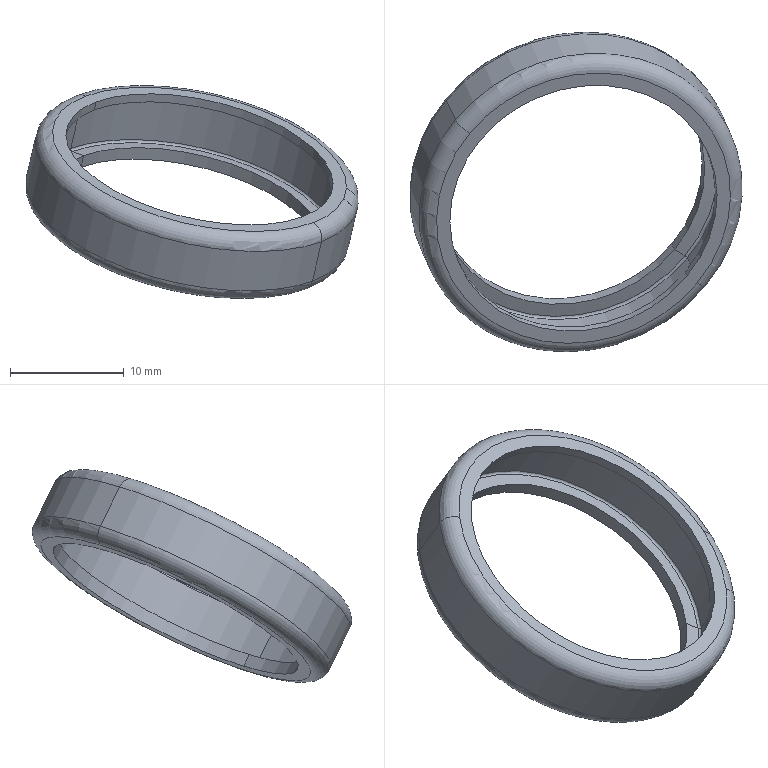Part | SolidWorks | features BaseBody 1 | 1 solid | 23 faces | box 29.254 x 28.081 x 18.745 mm | volume 719.848 mm3 | torus 10 | cylinder 8 | plane 3 | cone 2 | commonest cylinder face diameters 24 x4 27 x2 29 x2
STEP:
#1=CARTESIAN_POINT('',(1950.214,-223.457,971.31));
#2=VERTEX_POINT('',#1);
#3=CARTESIAN_POINT('',(1970.233,-236.588,960.184));
#4=VERTEX_POINT('',#3);
#5=CARTESIAN_POINT('',(1960.224,-230.022,965.747));
#6=DIRECTION('',(0.2015,-0.436,0.8771));
#7=DIRECTION('',(0.9077,0.4197,0.0001618));
#8=AXIS2_PLACEMENT_3D('',#5,#6,#7);
#9=CIRCLE('',#8,13.2);
#10=EDGE_CURVE('',#2,#4,#9,.T.);
#11=ORIENTED_EDGE('',*,*,#10,.F.);
#12=CARTESIAN_POINT('',(1948.967,-222.243,970.717));
#13=VERTEX_POINT('',#12);
#14=CARTESIAN_POINT('',(1949.952,-222.89,970.17));
#15=DIRECTION('',(0.62,0.75,0.2304));
#16=DIRECTION('',(0.7583,-0.4974,-0.4214));
#17=AXIS2_PLACEMENT_3D('',#14,#15,#16);
#18=CIRCLE('',#17,1.3);
#19=EDGE_CURVE('',#13,#2,#18,.T.);
#20=ORIENTED_EDGE('',*,*,#19,.F.);
#21=CARTESIAN_POINT('',(1970.957,-236.668,958.496));
#22=VERTEX_POINT('',#21);
#23=CARTESIAN_POINT('',(1959.962,-229.456,964.607));
#24=DIRECTION('',(0.2015,-0.436,0.8771));
#25=DIRECTION('',(0.9077,0.4197,0.0001618));
#26=AXIS2_PLACEMENT_3D('',#23,#24,#25);
#27=CIRCLE('',#26,14.5);
#28=EDGE_CURVE('',#13,#22,#27,.T.);
#29=ORIENTED_EDGE('',*,*,#28,.T.);
#30=CARTESIAN_POINT('',(1969.971,-236.021,959.044));
#31=DIRECTION('',(0.62,0.75,0.2304));
#32=DIRECTION('',(0.7583,-0.4974,-0.4214));
#33=AXIS2_PLACEMENT_3D('',#30,#31,#32);
#34=CIRCLE('',#33,1.3);
#35=EDGE_CURVE('',#4,#22,#34,.T.);
#36=ORIENTED_EDGE('',*,*,#35,.F.);
#37=EDGE_LOOP('',(#11,#20,#29,#36));
#38=FACE_OUTER_BOUND('',#37,.T.);
#39=CARTESIAN_POINT('',(1959.962,-229.456,964.607));
#40=DIRECTION('',(0.2015,-0.436,0.8771));
#41=DIRECTION('',(0.7583,-0.4974,-0.4214));
#42=AXIS2_PLACEMENT_3D('',#39,#40,#41);
#43=TOROIDAL_SURFACE('',#42,13.2,1.3);
#44=ADVANCED_FACE('',(#38),#43,.T.);
#45=CARTESIAN_POINT('',(1960.224,-230.022,965.747));
#46=DIRECTION('',(0.2015,-0.436,0.8771));
#47=DIRECTION('',(0.9077,0.4197,0.0001618));
#48=AXIS2_PLACEMENT_3D('',#45,#46,#47);
#49=CIRCLE('',#48,13.2);
#50=EDGE_CURVE('',#4,#2,#49,.T.);
#51=ORIENTED_EDGE('',*,*,#50,.F.);
#52=ORIENTED_EDGE('',*,*,#35,.T.);
#53=CARTESIAN_POINT('',(1959.962,-229.456,964.607));
#54=DIRECTION('',(0.2015,-0.436,0.8771));
#55=DIRECTION('',(0.9077,0.4197,0.0001618));
#56=AXIS2_PLACEMENT_3D('',#53,#54,#55);
#57=CIRCLE('',#56,14.5);
#58=EDGE_CURVE('',#22,#13,#57,.T.);
#59=ORIENTED_EDGE('',*,*,#58,.T.);
#60=ORIENTED_EDGE('',*,*,#19,.T.);
#61=EDGE_LOOP('',(#51,#52,#59,#60));
#62=FACE_OUTER_BOUND('',#61,.T.);
#63=CARTESIAN_POINT('',(1959.962,-229.456,964.607));
#64=DIRECTION('',(0.2015,-0.436,0.8771));
#65=DIRECTION('',(0.7583,-0.4974,-0.4214));
#66=AXIS2_PLACEMENT_3D('',#63,#64,#65);
#67=TOROIDAL_SURFACE('',#66,13.2,1.3);
#68=ADVANCED_FACE('',(#62),#67,.T.);
#69=ORIENTED_EDGE('',*,*,#28,.F.);
#70=CARTESIAN_POINT('',(1948.171,-220.521,967.253));
#71=VERTEX_POINT('',#70);
#72=CARTESIAN_POINT('',(1948.569,-221.382,968.985));
#73=DIRECTION('',(-0.2015,0.436,-0.8771));
#74=VECTOR('',#73,1000.);
#75=LINE('',#72,#74);
#76=EDGE_CURVE('',#13,#71,#75,.T.);
#77=ORIENTED_EDGE('',*,*,#76,.T.);
#78=CARTESIAN_POINT('',(1970.161,-234.946,955.031));
#79=VERTEX_POINT('',#78);
#80=CARTESIAN_POINT('',(1959.166,-227.733,961.142));
#81=DIRECTION('',(0.2015,-0.436,0.8771));
#82=DIRECTION('',(0.9077,0.4197,0.0001618));
#83=AXIS2_PLACEMENT_3D('',#80,#81,#82);
#84=CIRCLE('',#83,14.5);
#85=EDGE_CURVE('',#71,#79,#84,.T.);
#86=ORIENTED_EDGE('',*,*,#85,.T.);
#87=CARTESIAN_POINT('',(1970.559,-235.807,956.763));
#88=DIRECTION('',(0.2015,-0.436,0.8771));
#89=VECTOR('',#88,1000.);
#90=LINE('',#87,#89);
#91=EDGE_CURVE('',#79,#22,#90,.T.);
#92=ORIENTED_EDGE('',*,*,#91,.T.);
#93=EDGE_LOOP('',(#69,#77,#86,#92));
#94=FACE_OUTER_BOUND('',#93,.T.);
#95=CARTESIAN_POINT('',(1959.564,-228.595,962.874));
#96=DIRECTION('',(0.2015,-0.436,0.8771));
#97=DIRECTION('',(0.7583,-0.4974,-0.4214));
#98=AXIS2_PLACEMENT_3D('',#95,#96,#97);
#99=CYLINDRICAL_SURFACE('',#98,14.5);
#100=ADVANCED_FACE('',(#94),#99,.T.);
#101=ORIENTED_EDGE('',*,*,#58,.F.);
#102=ORIENTED_EDGE('',*,*,#91,.F.);
#103=CARTESIAN_POINT('',(1959.166,-227.733,961.142));
#104=DIRECTION('',(0.2015,-0.436,0.8771));
#105=DIRECTION('',(0.9077,0.4197,0.0001618));
#106=AXIS2_PLACEMENT_3D('',#103,#104,#105);
#107=CIRCLE('',#106,14.5);
#108=EDGE_CURVE('',#79,#71,#107,.T.);
#109=ORIENTED_EDGE('',*,*,#108,.T.);
#110=ORIENTED_EDGE('',*,*,#76,.F.);
#111=EDGE_LOOP('',(#101,#102,#109,#110));
#112=FACE_OUTER_BOUND('',#111,.T.);
#113=CARTESIAN_POINT('',(1959.564,-228.595,962.874));
#114=DIRECTION('',(0.2015,-0.436,0.8771));
#115=DIRECTION('',(0.7583,-0.4974,-0.4214));
#116=AXIS2_PLACEMENT_3D('',#113,#114,#115);
#117=CYLINDRICAL_SURFACE('',#116,14.5);
#118=ADVANCED_FACE('',(#112),#117,.T.);
#119=ORIENTED_EDGE('',*,*,#85,.F.);
#120=CARTESIAN_POINT('',(1948.895,-220.601,965.565));
#121=VERTEX_POINT('',#120);
#122=CARTESIAN_POINT('',(1949.157,-221.168,966.705));
#123=DIRECTION('',(-0.62,-0.75,-0.2304));
#124=DIRECTION('',(0.7583,-0.4974,-0.4214));
#125=AXIS2_PLACEMENT_3D('',#122,#123,#124);
#126=CIRCLE('',#125,1.3);
#127=EDGE_CURVE('',#71,#121,#126,.T.);
#128=ORIENTED_EDGE('',*,*,#127,.T.);
#129=CARTESIAN_POINT('',(1968.913,-233.732,954.439));
#130=VERTEX_POINT('',#129);
#131=CARTESIAN_POINT('',(1958.904,-227.167,960.002));
#132=DIRECTION('',(0.2015,-0.436,0.8771));
#133=DIRECTION('',(0.9077,0.4197,0.0001618));
#134=AXIS2_PLACEMENT_3D('',#131,#132,#133);
#135=CIRCLE('',#134,13.2);
#136=EDGE_CURVE('',#121,#130,#135,.T.);
#137=ORIENTED_EDGE('',*,*,#136,.T.);
#138=CARTESIAN_POINT('',(1969.175,-234.299,955.579));
#139=DIRECTION('',(-0.62,-0.75,-0.2304));
#140=DIRECTION('',(0.7583,-0.4974,-0.4214));
#141=AXIS2_PLACEMENT_3D('',#138,#139,#140);
#142=CIRCLE('',#141,1.3);
#143=EDGE_CURVE('',#130,#79,#142,.T.);
#144=ORIENTED_EDGE('',*,*,#143,.T.);
#145=EDGE_LOOP('',(#119,#128,#137,#144));
#146=FACE_OUTER_BOUND('',#145,.T.);
#147=CARTESIAN_POINT('',(1959.166,-227.733,961.142));
#148=DIRECTION('',(0.2015,-0.436,0.8771));
#149=DIRECTION('',(0.7583,-0.4974,-0.4214));
#150=AXIS2_PLACEMENT_3D('',#147,#148,#149);
#151=TOROIDAL_SURFACE('',#150,13.2,1.3);
#152=ADVANCED_FACE('',(#146),#151,.T.);
#153=ORIENTED_EDGE('',*,*,#108,.F.);
#154=ORIENTED_EDGE('',*,*,#143,.F.);
#155=CARTESIAN_POINT('',(1958.904,-227.167,960.002));
#156=DIRECTION('',(0.2015,-0.436,0.8771));
#157=DIRECTION('',(0.9077,0.4197,0.0001618));
#158=AXIS2_PLACEMENT_3D('',#155,#156,#157);
#159=CIRCLE('',#158,13.2);
#160=EDGE_CURVE('',#130,#121,#159,.T.);
#161=ORIENTED_EDGE('',*,*,#160,.T.);
#162=ORIENTED_EDGE('',*,*,#127,.F.);
#163=EDGE_LOOP('',(#153,#154,#161,#162));
#164=FACE_OUTER_BOUND('',#163,.T.);
#165=CARTESIAN_POINT('',(1959.166,-227.733,961.142));
#166=DIRECTION('',(0.2015,-0.436,0.8771));
#167=DIRECTION('',(0.7583,-0.4974,-0.4214));
#168=AXIS2_PLACEMENT_3D('',#165,#166,#167);
#169=TOROIDAL_SURFACE('',#168,13.2,1.3);
#170=ADVANCED_FACE('',(#164),#169,.T.);
#171=CARTESIAN_POINT('',(1949.805,-221.198,965.059));
#172=VERTEX_POINT('',#171);
#173=CARTESIAN_POINT('',(1968.004,-233.135,954.945));
#174=VERTEX_POINT('',#173);
#175=CARTESIAN_POINT('',(1958.904,-227.167,960.002));
#176=DIRECTION('',(0.2015,-0.436,0.8771));
#177=DIRECTION('',(0.9077,0.4197,0.0001618));
#178=AXIS2_PLACEMENT_3D('',#175,#176,#177);
#179=CIRCLE('',#178,12.);
#180=EDGE_CURVE('',#172,#174,#179,.T.);
#181=ORIENTED_EDGE('',*,*,#180,.F.);
#182=CARTESIAN_POINT('',(1950.036,-221.699,966.068));
#183=VERTEX_POINT('',#182);
#184=CARTESIAN_POINT('',(1950.465,-222.626,967.932));
#185=DIRECTION('',(0.2015,-0.436,0.8771));
#186=VECTOR('',#185,1000.);
#187=LINE('',#184,#186);
#188=EDGE_CURVE('',#172,#183,#187,.T.);
#189=ORIENTED_EDGE('',*,*,#188,.T.);
#190=CARTESIAN_POINT('',(1968.235,-233.637,955.953));
#191=VERTEX_POINT('',#190);
#192=CARTESIAN_POINT('',(1959.136,-227.668,961.01));
#193=DIRECTION('',(0.2015,-0.436,0.8771));
#194=DIRECTION('',(0.9077,0.4197,0.0001618));
#195=AXIS2_PLACEMENT_3D('',#192,#193,#194);
#196=CIRCLE('',#195,12.);
#197=EDGE_CURVE('',#183,#191,#196,.T.);
#198=ORIENTED_EDGE('',*,*,#197,.T.);
#199=CARTESIAN_POINT('',(1968.663,-234.563,957.817));
#200=DIRECTION('',(-0.2015,0.436,-0.8771));
#201=VECTOR('',#200,1000.);
#202=LINE('',#199,#201);
#203=EDGE_CURVE('',#191,#174,#202,.T.);
#204=ORIENTED_EDGE('',*,*,#203,.T.);
#205=EDGE_LOOP('',(#181,#189,#198,#204));
#206=FACE_OUTER_BOUND('',#205,.T.);
#207=CARTESIAN_POINT('',(1959.564,-228.595,962.874));
#208=DIRECTION('',(0.2015,-0.436,0.8771));
#209=DIRECTION('',(0.7583,-0.4974,-0.4214));
#210=AXIS2_PLACEMENT_3D('',#207,#208,#209);
#211=CYLINDRICAL_SURFACE('',#210,12.);
#212=ADVANCED_FACE('',(#206),#211,.F.);
#213=CARTESIAN_POINT('',(1958.904,-227.167,960.002));
#214=DIRECTION('',(0.2015,-0.436,0.8771));
#215=DIRECTION('',(0.9077,0.4197,0.0001618));
#216=AXIS2_PLACEMENT_3D('',#213,#214,#215);
#217=CIRCLE('',#216,12.);
#218=EDGE_CURVE('',#174,#172,#217,.T.);
#219=ORIENTED_EDGE('',*,*,#218,.F.);
#220=ORIENTED_EDGE('',*,*,#203,.F.);
#221=CARTESIAN_POINT('',(1959.136,-227.668,961.01));
#222=DIRECTION('',(0.2015,-0.436,0.8771));
#223=DIRECTION('',(0.9077,0.4197,0.0001618));
#224=AXIS2_PLACEMENT_3D('',#221,#222,#223);
#225=CIRCLE('',#224,12.);
#226=EDGE_CURVE('',#191,#183,#225,.T.);
#227=ORIENTED_EDGE('',*,*,#226,.T.);
#228=ORIENTED_EDGE('',*,*,#188,.F.);
#229=EDGE_LOOP('',(#219,#220,#227,#228));
#230=FACE_OUTER_BOUND('',#229,.T.);
#231=CARTESIAN_POINT('',(1959.564,-228.595,962.874));
#232=DIRECTION('',(0.2015,-0.436,0.8771));
#233=DIRECTION('',(0.7583,-0.4974,-0.4214));
#234=AXIS2_PLACEMENT_3D('',#231,#232,#233);
#235=CYLINDRICAL_SURFACE('',#234,12.);
#236=ADVANCED_FACE('',(#230),#235,.F.);
#237=ORIENTED_EDGE('',*,*,#197,.F.);
#238=CARTESIAN_POINT('',(1949.034,-220.982,966.429));
#239=VERTEX_POINT('',#238);
#240=CARTESIAN_POINT('',(1949.535,-221.341,966.248));
#241=DIRECTION('',(0.7803,-0.5585,-0.2815));
#242=VECTOR('',#241,1000.);
#243=LINE('',#240,#242);
#244=EDGE_CURVE('',#239,#183,#243,.T.);
#245=ORIENTED_EDGE('',*,*,#244,.F.);
#246=CARTESIAN_POINT('',(1969.158,-234.182,955.245));
#247=VERTEX_POINT('',#246);
#248=CARTESIAN_POINT('',(1959.096,-227.582,960.837));
#249=DIRECTION('',(0.2015,-0.436,0.8771));
#250=DIRECTION('',(0.9077,0.4197,0.0001618));
#251=AXIS2_PLACEMENT_3D('',#248,#249,#250);
#252=CIRCLE('',#251,13.269);
#253=EDGE_CURVE('',#239,#247,#252,.T.);
#254=ORIENTED_EDGE('',*,*,#253,.T.);
#255=CARTESIAN_POINT('',(1968.697,-233.909,955.599));
#256=DIRECTION('',(0.7183,-0.4244,-0.5514));
#257=VECTOR('',#256,1000.);
#258=LINE('',#255,#257);
#259=EDGE_CURVE('',#191,#247,#258,.T.);
#260=ORIENTED_EDGE('',*,*,#259,.F.);
#261=EDGE_LOOP('',(#237,#245,#254,#260));
#262=FACE_OUTER_BOUND('',#261,.T.);
#263=CARTESIAN_POINT('',(1959.136,-227.668,961.01));
#264=DIRECTION('',(-0.2015,0.436,-0.8771));
#265=DIRECTION('',(0.7583,-0.4974,-0.4214));
#266=AXIS2_PLACEMENT_3D('',#263,#264,#265);
#267=CONICAL_SURFACE('',#266,12.,1.416);
#268=ADVANCED_FACE('',(#262),#267,.T.);
#269=ORIENTED_EDGE('',*,*,#226,.F.);
#270=ORIENTED_EDGE('',*,*,#259,.T.);
#271=CARTESIAN_POINT('',(1959.096,-227.582,960.837));
#272=DIRECTION('',(0.2015,-0.436,0.8771));
#273=DIRECTION('',(0.9077,0.4197,0.0001618));
#274=AXIS2_PLACEMENT_3D('',#271,#272,#273);
#275=CIRCLE('',#274,13.269);
#276=EDGE_CURVE('',#247,#239,#275,.T.);
#277=ORIENTED_EDGE('',*,*,#276,.T.);
#278=ORIENTED_EDGE('',*,*,#244,.T.);
#279=EDGE_LOOP('',(#269,#270,#277,#278));
#280=FACE_OUTER_BOUND('',#279,.T.);
#281=CARTESIAN_POINT('',(1959.136,-227.668,961.01));
#282=DIRECTION('',(-0.2015,0.436,-0.8771));
#283=DIRECTION('',(0.7583,-0.4974,-0.4214));
#284=AXIS2_PLACEMENT_3D('',#281,#282,#283);
#285=CONICAL_SURFACE('',#284,12.,1.416);
#286=ADVANCED_FACE('',(#280),#285,.T.);
#287=ORIENTED_EDGE('',*,*,#253,.F.);
#288=CARTESIAN_POINT('',(1948.899,-220.953,966.7));
#289=VERTEX_POINT('',#288);
#290=CARTESIAN_POINT('',(1949.051,-221.053,966.616));
#291=DIRECTION('',(0.62,0.75,0.2304));
#292=DIRECTION('',(0.7583,-0.4974,-0.4214));
#293=AXIS2_PLACEMENT_3D('',#290,#291,#292);
#294=CIRCLE('',#293,0.2);
#295=EDGE_CURVE('',#239,#289,#294,.T.);
#296=ORIENTED_EDGE('',*,*,#295,.T.);
#297=CARTESIAN_POINT('',(1969.373,-234.383,955.321));
#298=VERTEX_POINT('',#297);
#299=CARTESIAN_POINT('',(1959.136,-227.668,961.01));
#300=DIRECTION('',(0.2015,-0.436,0.8771));
#301=DIRECTION('',(0.9077,0.4197,0.0001618));
#302=AXIS2_PLACEMENT_3D('',#299,#300,#301);
#303=CIRCLE('',#302,13.5);
#304=EDGE_CURVE('',#289,#298,#303,.T.);
#305=ORIENTED_EDGE('',*,*,#304,.T.);
#306=CARTESIAN_POINT('',(1969.221,-234.283,955.405));
#307=DIRECTION('',(0.62,0.75,0.2304));
#308=DIRECTION('',(0.7583,-0.4974,-0.4214));
#309=AXIS2_PLACEMENT_3D('',#306,#307,#308);
#310=CIRCLE('',#309,0.2);
#311=EDGE_CURVE('',#298,#247,#310,.T.);
#312=ORIENTED_EDGE('',*,*,#311,.T.);
#313=EDGE_LOOP('',(#287,#296,#305,#312));
#314=FACE_OUTER_BOUND('',#313,.T.);
#315=CARTESIAN_POINT('',(1959.136,-227.668,961.01));
#316=DIRECTION('',(0.2015,-0.436,0.8771));
#317=DIRECTION('',(0.7583,-0.4974,-0.4214));
#318=AXIS2_PLACEMENT_3D('',#315,#316,#317);
#319=TOROIDAL_SURFACE('',#318,13.3,0.2);
#320=ADVANCED_FACE('',(#314),#319,.F.);
#321=ORIENTED_EDGE('',*,*,#276,.F.);
#322=ORIENTED_EDGE('',*,*,#311,.F.);
#323=CARTESIAN_POINT('',(1959.136,-227.668,961.01));
#324=DIRECTION('',(0.2015,-0.436,0.8771));
#325=DIRECTION('',(0.9077,0.4197,0.0001618));
#326=AXIS2_PLACEMENT_3D('',#323,#324,#325);
#327=CIRCLE('',#326,13.5);
#328=EDGE_CURVE('',#298,#289,#327,.T.);
#329=ORIENTED_EDGE('',*,*,#328,.T.);
#330=ORIENTED_EDGE('',*,*,#295,.F.);
#331=EDGE_LOOP('',(#321,#322,#329,#330));
#332=FACE_OUTER_BOUND('',#331,.T.);
#333=CARTESIAN_POINT('',(1959.136,-227.668,961.01));
#334=DIRECTION('',(0.2015,-0.436,0.8771));
#335=DIRECTION('',(0.7583,-0.4974,-0.4214));
#336=AXIS2_PLACEMENT_3D('',#333,#334,#335);
#337=TOROIDAL_SURFACE('',#336,13.3,0.2);
#338=ADVANCED_FACE('',(#332),#337,.F.);
#339=ORIENTED_EDGE('',*,*,#304,.F.);
#340=CARTESIAN_POINT('',(1949.685,-222.654,970.121));
#341=VERTEX_POINT('',#340);
#342=CARTESIAN_POINT('',(1949.292,-221.803,968.41));
#343=DIRECTION('',(-0.2015,0.436,-0.8771));
#344=VECTOR('',#343,1000.);
#345=LINE('',#342,#344);
#346=EDGE_CURVE('',#341,#289,#345,.T.);
#347=ORIENTED_EDGE('',*,*,#346,.F.);
#348=CARTESIAN_POINT('',(1970.158,-236.083,958.742));
#349=VERTEX_POINT('',#348);
#350=CARTESIAN_POINT('',(1959.922,-229.368,964.431));
#351=DIRECTION('',(0.2015,-0.436,0.8771));
#352=DIRECTION('',(0.9077,0.4197,0.0001618));
#353=AXIS2_PLACEMENT_3D('',#350,#351,#352);
#354=CIRCLE('',#353,13.5);
#355=EDGE_CURVE('',#341,#349,#354,.T.);
#356=ORIENTED_EDGE('',*,*,#355,.T.);
#357=CARTESIAN_POINT('',(1969.765,-235.233,957.031));
#358=DIRECTION('',(0.2015,-0.436,0.8771));
#359=VECTOR('',#358,1000.);
#360=LINE('',#357,#359);
#361=EDGE_CURVE('',#298,#349,#360,.T.);
#362=ORIENTED_EDGE('',*,*,#361,.F.);
#363=EDGE_LOOP('',(#339,#347,#356,#362));
#364=FACE_OUTER_BOUND('',#363,.T.);
#365=CARTESIAN_POINT('',(1959.564,-228.595,962.874));
#366=DIRECTION('',(0.2015,-0.436,0.8771));
#367=DIRECTION('',(0.7583,-0.4974,-0.4214));
#368=AXIS2_PLACEMENT_3D('',#365,#366,#367);
#369=CYLINDRICAL_SURFACE('',#368,13.5);
#370=ADVANCED_FACE('',(#364),#369,.F.);
#371=ORIENTED_EDGE('',*,*,#328,.F.);
#372=ORIENTED_EDGE('',*,*,#361,.T.);
#373=CARTESIAN_POINT('',(1959.922,-229.368,964.431));
#374=DIRECTION('',(0.2015,-0.436,0.8771));
#375=DIRECTION('',(0.9077,0.4197,0.0001618));
#376=AXIS2_PLACEMENT_3D('',#373,#374,#375);
#377=CIRCLE('',#376,13.5);
#378=EDGE_CURVE('',#349,#341,#377,.T.);
#379=ORIENTED_EDGE('',*,*,#378,.T.);
#380=ORIENTED_EDGE('',*,*,#346,.T.);
#381=EDGE_LOOP('',(#371,#372,#379,#380));
#382=FACE_OUTER_BOUND('',#381,.T.);
#383=CARTESIAN_POINT('',(1959.564,-228.595,962.874));
#384=DIRECTION('',(0.2015,-0.436,0.8771));
#385=DIRECTION('',(0.7583,-0.4974,-0.4214));
#386=AXIS2_PLACEMENT_3D('',#383,#384,#385);
#387=CYLINDRICAL_SURFACE('',#386,13.5);
#388=ADVANCED_FACE('',(#382),#387,.F.);
#389=ORIENTED_EDGE('',*,*,#355,.F.);
#390=CARTESIAN_POINT('',(1949.585,-222.635,970.329));
#391=VERTEX_POINT('',#390);
#392=CARTESIAN_POINT('',(1948.983,-221.992,969.855));
#393=DIRECTION('',(-0.62,-0.75,-0.2304));
#394=DIRECTION('',(0.7583,-0.4974,-0.4214));
#395=AXIS2_PLACEMENT_3D('',#392,#393,#394);
#396=CIRCLE('',#395,1.);
#397=EDGE_CURVE('',#341,#391,#396,.T.);
#398=ORIENTED_EDGE('',*,*,#397,.T.);
#399=CARTESIAN_POINT('',(1970.321,-236.237,958.805));
#400=VERTEX_POINT('',#399);
#401=CARTESIAN_POINT('',(1959.953,-229.436,964.567));
#402=DIRECTION('',(0.2015,-0.436,0.8771));
#403=DIRECTION('',(0.9077,0.4197,0.0001618));
#404=AXIS2_PLACEMENT_3D('',#401,#402,#403);
#405=CIRCLE('',#404,13.673);
#406=EDGE_CURVE('',#391,#400,#405,.T.);
#407=ORIENTED_EDGE('',*,*,#406,.T.);
#408=CARTESIAN_POINT('',(1970.593,-236.167,957.845));
#409=DIRECTION('',(-0.62,-0.75,-0.2304));
#410=DIRECTION('',(0.7583,-0.4974,-0.4214));
#411=AXIS2_PLACEMENT_3D('',#408,#409,#410);
#412=CIRCLE('',#411,1.);
#413=EDGE_CURVE('',#400,#349,#412,.T.);
#414=ORIENTED_EDGE('',*,*,#413,.T.);
#415=EDGE_LOOP('',(#389,#398,#407,#414));
#416=FACE_OUTER_BOUND('',#415,.T.);
#417=CARTESIAN_POINT('',(1959.788,-229.08,963.85));
#418=DIRECTION('',(0.2015,-0.436,0.8771));
#419=DIRECTION('',(0.7583,-0.4974,-0.4214));
#420=AXIS2_PLACEMENT_3D('',#417,#418,#419);
#421=TOROIDAL_SURFACE('',#420,14.249,1.);
#422=ADVANCED_FACE('',(#416),#421,.T.);
#423=ORIENTED_EDGE('',*,*,#378,.F.);
#424=ORIENTED_EDGE('',*,*,#413,.F.);
#425=CARTESIAN_POINT('',(1959.953,-229.436,964.567));
#426=DIRECTION('',(0.2015,-0.436,0.8771));
#427=DIRECTION('',(0.9077,0.4197,0.0001618));
#428=AXIS2_PLACEMENT_3D('',#425,#426,#427);
#429=CIRCLE('',#428,13.673);
#430=EDGE_CURVE('',#400,#391,#429,.T.);
#431=ORIENTED_EDGE('',*,*,#430,.T.);
#432=ORIENTED_EDGE('',*,*,#397,.F.);
#433=EDGE_LOOP('',(#423,#424,#431,#432));
#434=FACE_OUTER_BOUND('',#433,.T.);
#435=CARTESIAN_POINT('',(1959.788,-229.08,963.85));
#436=DIRECTION('',(0.2015,-0.436,0.8771));
#437=DIRECTION('',(0.7583,-0.4974,-0.4214));
#438=AXIS2_PLACEMENT_3D('',#435,#436,#437);
#439=TOROIDAL_SURFACE('',#438,14.249,1.);
#440=ADVANCED_FACE('',(#434),#439,.T.);
#441=ORIENTED_EDGE('',*,*,#406,.F.);
#442=CARTESIAN_POINT('',(1949.826,-222.959,970.735));
#443=VERTEX_POINT('',#442);
#444=CARTESIAN_POINT('',(1949.765,-222.828,970.471));
#445=DIRECTION('',(0.62,0.75,0.2304));
#446=DIRECTION('',(0.7583,-0.4974,-0.4214));
#447=AXIS2_PLACEMENT_3D('',#444,#445,#446);
#448=CIRCLE('',#447,0.3);
#449=EDGE_CURVE('',#391,#443,#448,.T.);
#450=ORIENTED_EDGE('',*,*,#449,.T.);
#451=CARTESIAN_POINT('',(1970.299,-236.388,959.356));
#452=VERTEX_POINT('',#451);
#453=CARTESIAN_POINT('',(1960.063,-229.674,965.045));
#454=DIRECTION('',(0.2015,-0.436,0.8771));
#455=DIRECTION('',(0.9077,0.4197,0.0001618));
#456=AXIS2_PLACEMENT_3D('',#453,#454,#455);
#457=CIRCLE('',#456,13.5);
#458=EDGE_CURVE('',#443,#452,#457,.T.);
#459=ORIENTED_EDGE('',*,*,#458,.T.);
#460=CARTESIAN_POINT('',(1970.239,-236.258,959.093));
#461=DIRECTION('',(0.62,0.75,0.2304));
#462=DIRECTION('',(0.7583,-0.4974,-0.4214));
#463=AXIS2_PLACEMENT_3D('',#460,#461,#462);
#464=CIRCLE('',#463,0.3);
#465=EDGE_CURVE('',#452,#400,#464,.T.);
#466=ORIENTED_EDGE('',*,*,#465,.T.);
#467=EDGE_LOOP('',(#441,#450,#459,#466));
#468=FACE_OUTER_BOUND('',#467,.T.);
#469=CARTESIAN_POINT('',(1960.002,-229.543,964.782));
#470=DIRECTION('',(0.2015,-0.436,0.8771));
#471=DIRECTION('',(0.7583,-0.4974,-0.4214));
#472=AXIS2_PLACEMENT_3D('',#469,#470,#471);
#473=TOROIDAL_SURFACE('',#472,13.5,0.3);
#474=ADVANCED_FACE('',(#468),#473,.F.);
#475=ORIENTED_EDGE('',*,*,#430,.F.);
#476=ORIENTED_EDGE('',*,*,#465,.F.);
#477=CARTESIAN_POINT('',(1960.063,-229.674,965.045));
#478=DIRECTION('',(0.2015,-0.436,0.8771));
#479=DIRECTION('',(0.9077,0.4197,0.0001618));
#480=AXIS2_PLACEMENT_3D('',#477,#478,#479);
#481=CIRCLE('',#480,13.5);
#482=EDGE_CURVE('',#452,#443,#481,.T.);
#483=ORIENTED_EDGE('',*,*,#482,.T.);
#484=ORIENTED_EDGE('',*,*,#449,.F.);
#485=EDGE_LOOP('',(#475,#476,#483,#484));
#486=FACE_OUTER_BOUND('',#485,.T.);
#487=CARTESIAN_POINT('',(1960.002,-229.543,964.782));
#488=DIRECTION('',(0.2015,-0.436,0.8771));
#489=DIRECTION('',(0.7583,-0.4974,-0.4214));
#490=AXIS2_PLACEMENT_3D('',#487,#488,#489);
#491=TOROIDAL_SURFACE('',#490,13.5,0.3);
#492=ADVANCED_FACE('',(#486),#491,.F.);
#493=CARTESIAN_POINT('',(1950.963,-223.705,970.102));
#494=VERTEX_POINT('',#493);
#495=CARTESIAN_POINT('',(1969.162,-235.642,959.988));
#496=VERTEX_POINT('',#495);
#497=CARTESIAN_POINT('',(1960.063,-229.674,965.045));
#498=DIRECTION('',(0.2015,-0.436,0.8771));
#499=DIRECTION('',(0.9077,0.4197,0.0001618));
#500=AXIS2_PLACEMENT_3D('',#497,#498,#499);
#501=CIRCLE('',#500,12.);
#502=EDGE_CURVE('',#494,#496,#501,.T.);
#503=ORIENTED_EDGE('',*,*,#502,.F.);
#504=CARTESIAN_POINT('',(1951.124,-224.054,970.804));
#505=VERTEX_POINT('',#504);
#506=CARTESIAN_POINT('',(1950.465,-222.626,967.932));
#507=DIRECTION('',(-0.2015,0.436,-0.8771));
#508=VECTOR('',#507,1000.);
#509=LINE('',#506,#508);
#510=EDGE_CURVE('',#505,#494,#509,.T.);
#511=ORIENTED_EDGE('',*,*,#510,.F.);
#512=CARTESIAN_POINT('',(1969.323,-235.991,960.69));
#513=VERTEX_POINT('',#512);
#514=CARTESIAN_POINT('',(1960.224,-230.022,965.747));
#515=DIRECTION('',(0.2015,-0.436,0.8771));
#516=DIRECTION('',(0.9077,0.4197,0.0001618));
#517=AXIS2_PLACEMENT_3D('',#514,#515,#516);
#518=CIRCLE('',#517,12.);
#519=EDGE_CURVE('',#505,#513,#518,.T.);
#520=ORIENTED_EDGE('',*,*,#519,.T.);
#521=CARTESIAN_POINT('',(1968.663,-234.563,957.817));
#522=DIRECTION('',(0.2015,-0.436,0.8771));
#523=VECTOR('',#522,1000.);
#524=LINE('',#521,#523);
#525=EDGE_CURVE('',#496,#513,#524,.T.);
#526=ORIENTED_EDGE('',*,*,#525,.F.);
#527=EDGE_LOOP('',(#503,#511,#520,#526));
#528=FACE_OUTER_BOUND('',#527,.T.);
#529=CARTESIAN_POINT('',(1959.564,-228.595,962.874));
#530=DIRECTION('',(0.2015,-0.436,0.8771));
#531=DIRECTION('',(0.7583,-0.4974,-0.4214));
#532=AXIS2_PLACEMENT_3D('',#529,#530,#531);
#533=CYLINDRICAL_SURFACE('',#532,12.);
#534=ADVANCED_FACE('',(#528),#533,.F.);
#535=CARTESIAN_POINT('',(1960.063,-229.674,965.045));
#536=DIRECTION('',(0.2015,-0.436,0.8771));
#537=DIRECTION('',(0.9077,0.4197,0.0001618));
#538=AXIS2_PLACEMENT_3D('',#535,#536,#537);
#539=CIRCLE('',#538,12.);
#540=EDGE_CURVE('',#496,#494,#539,.T.);
#541=ORIENTED_EDGE('',*,*,#540,.F.);
#542=ORIENTED_EDGE('',*,*,#525,.T.);
#543=CARTESIAN_POINT('',(1960.224,-230.022,965.747));
#544=DIRECTION('',(0.2015,-0.436,0.8771));
#545=DIRECTION('',(0.9077,0.4197,0.0001618));
#546=AXIS2_PLACEMENT_3D('',#543,#544,#545);
#547=CIRCLE('',#546,12.);
#548=EDGE_CURVE('',#513,#505,#547,.T.);
#549=ORIENTED_EDGE('',*,*,#548,.T.);
#550=ORIENTED_EDGE('',*,*,#510,.T.);
#551=EDGE_LOOP('',(#541,#542,#549,#550));
#552=FACE_OUTER_BOUND('',#551,.T.);
#553=CARTESIAN_POINT('',(1959.564,-228.595,962.874));
#554=DIRECTION('',(0.2015,-0.436,0.8771));
#555=DIRECTION('',(0.7583,-0.4974,-0.4214));
#556=AXIS2_PLACEMENT_3D('',#553,#554,#555);
#557=CYLINDRICAL_SURFACE('',#556,12.);
#558=ADVANCED_FACE('',(#552),#557,.F.);
#559=ORIENTED_EDGE('',*,*,#136,.F.);
#560=ORIENTED_EDGE('',*,*,#160,.F.);
#561=EDGE_LOOP('',(#559,#560));
#562=FACE_OUTER_BOUND('',#561,.T.);
#563=ORIENTED_EDGE('',*,*,#218,.T.);
#564=ORIENTED_EDGE('',*,*,#180,.T.);
#565=EDGE_LOOP('',(#563,#564));
#566=FACE_BOUND('',#565,.T.);
#567=CARTESIAN_POINT('',(1954.044,-216.658,966.342));
#568=DIRECTION('',(0.2015,-0.436,0.8771));
#569=DIRECTION('',(-0.9077,-0.4197,-0.0001618));
#570=AXIS2_PLACEMENT_3D('',#567,#568,#569);
#571=PLANE('',#570);
#572=ADVANCED_FACE('',(#562,#566),#571,.F.);
#573=ORIENTED_EDGE('',*,*,#458,.F.);
#574=ORIENTED_EDGE('',*,*,#482,.F.);
#575=EDGE_LOOP('',(#573,#574));
#576=FACE_OUTER_BOUND('',#575,.T.);
#577=ORIENTED_EDGE('',*,*,#540,.T.);
#578=ORIENTED_EDGE('',*,*,#502,.T.);
#579=EDGE_LOOP('',(#577,#578));
#580=FACE_BOUND('',#579,.T.);
#581=CARTESIAN_POINT('',(1955.644,-220.121,970.809));
#582=DIRECTION('',(0.2015,-0.436,0.8771));
#583=DIRECTION('',(-0.9077,-0.4197,-0.0001618));
#584=AXIS2_PLACEMENT_3D('',#581,#582,#583);
#585=PLANE('',#584);
#586=ADVANCED_FACE('',(#576,#580),#585,.F.);
#587=ORIENTED_EDGE('',*,*,#50,.T.);
#588=ORIENTED_EDGE('',*,*,#10,.T.);
#589=EDGE_LOOP('',(#587,#588));
#590=FACE_OUTER_BOUND('',#589,.T.);
#591=ORIENTED_EDGE('',*,*,#519,.F.);
#592=ORIENTED_EDGE('',*,*,#548,.F.);
#593=EDGE_LOOP('',(#591,#592));
#594=FACE_BOUND('',#593,.T.);
#595=CARTESIAN_POINT('',(1955.363,-219.514,972.087));
#596=DIRECTION('',(0.2015,-0.436,0.8771));
#597=DIRECTION('',(-0.9077,-0.4197,-0.0001618));
#598=AXIS2_PLACEMENT_3D('',#595,#596,#597);
#599=PLANE('',#598);
#600=ADVANCED_FACE('',(#590,#594),#599,.T.);
#601=CLOSED_SHELL('',(#44,#68,#100,#118,#152,#170,#212,#236,#268,#286,#320,#338,#370,#388,#422,#440,#474,#492,#534,#558,#572,#586,#600));
#602=MANIFOLD_SOLID_BREP('',#601);
#603=CARTESIAN_POINT('',(0.,0.,0.));
#604=DIRECTION('',(0.,0.,1.));
#605=DIRECTION('',(1.,0.,0.));
#606=AXIS2_PLACEMENT_3D('',#603,#604,#605);
#607=(LENGTH_UNIT()NAMED_UNIT(*)SI_UNIT(.MILLI.,.METRE.));
#608=UNCERTAINTY_MEASURE_WITH_UNIT(LENGTH_MEASURE(0.00001),#607,'','');
#609=(NAMED_UNIT(*)PLANE_ANGLE_UNIT()SI_UNIT($,.RADIAN.));
#610=(NAMED_UNIT(*)SI_UNIT($,.STERADIAN.)SOLID_ANGLE_UNIT());
#611=(GEOMETRIC_REPRESENTATION_CONTEXT(3)GLOBAL_UNCERTAINTY_ASSIGNED_CONTEXT((#608))GLOBAL_UNIT_ASSIGNED_CONTEXT((#607,#609,#610))REPRESENTATION_CONTEXT('',''));
#612=ADVANCED_BREP_SHAPE_REPRESENTATION('',(#602,#606),#611);